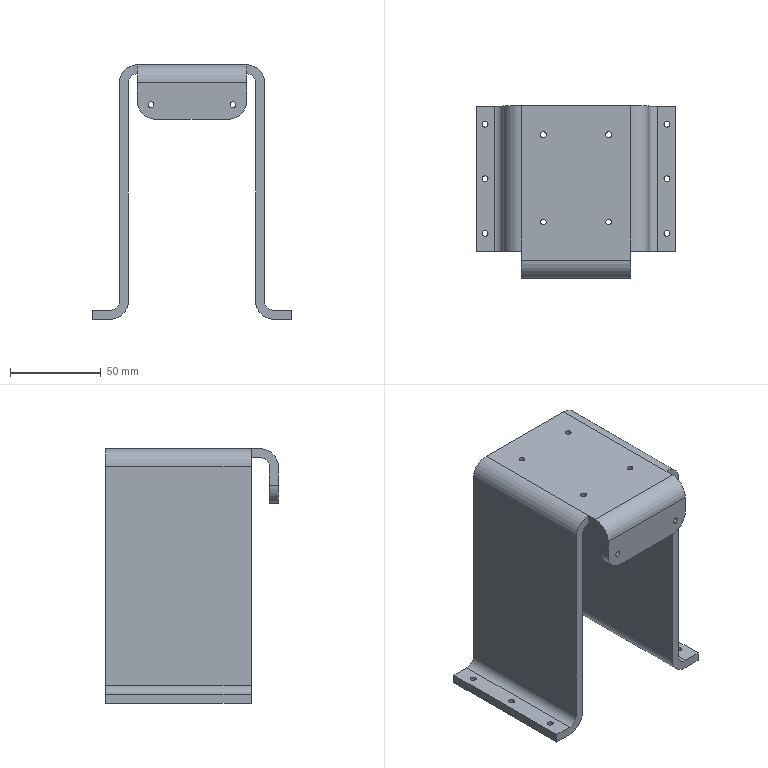Part | SolidWorks | features ICE 7, Fillet 5, Extrusion 1 | 1 solid | 56 faces | box 110 x 95 x 140 mm | volume 157187 mm3 | cylinder 36 | plane 20 | commonest cylinder face diameters 3.2 x24 20 x7 10 x5